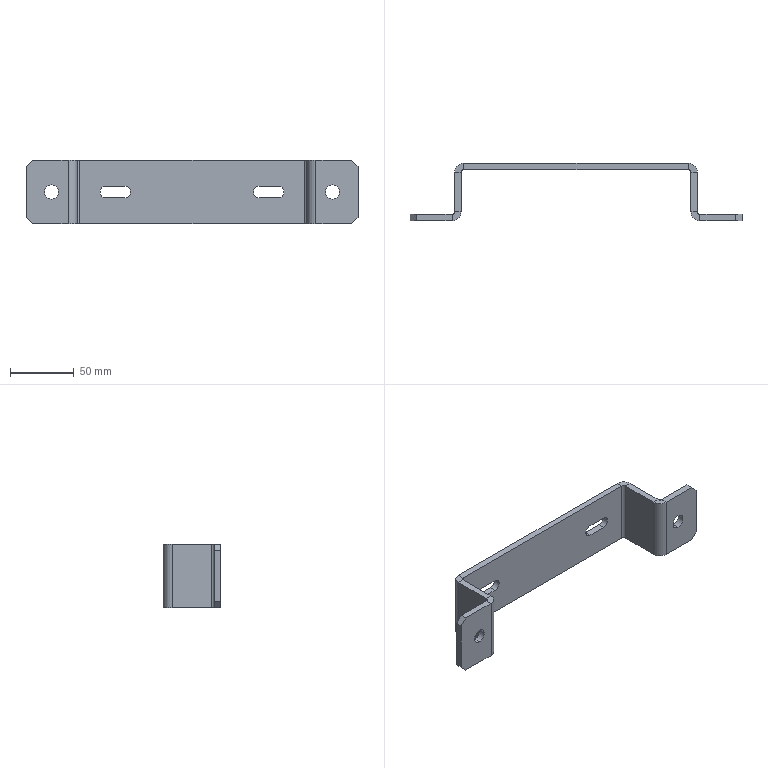Part | SolidWorks | features ICE 2, Chamfer 1, FlatPattern 1, SMBaseFlange 1, SheetMetal 1 | 1 solid | 54 faces | box 260 x 45 x 50 mm | volume 79882 mm3 | plane 38 | cylinder 16 | commonest cylinder face diameters 4 x4 9 x4 11 x4 14 x4
STEP:
#1=CARTESIAN_POINT('',(110.,0.,19.5));
#2=VERTEX_POINT('',#1);
#3=CARTESIAN_POINT('',(110.,0.,30.5));
#4=VERTEX_POINT('',#3);
#5=CARTESIAN_POINT('',(110.,0.,25.));
#6=DIRECTION('',(0.,1.,0.));
#7=DIRECTION('',(0.,0.,1.));
#8=AXIS2_PLACEMENT_3D('',#5,#6,#7);
#9=CIRCLE('',#8,5.5);
#10=EDGE_CURVE('',#2,#4,#9,.T.);
#11=ORIENTED_EDGE('',*,*,#10,.F.);
#12=CARTESIAN_POINT('',(110.,5.,19.5));
#13=VERTEX_POINT('',#12);
#14=CARTESIAN_POINT('',(110.,0.,19.5));
#15=DIRECTION('',(0.,1.,0.));
#16=VECTOR('',#15,1000.);
#17=LINE('',#14,#16);
#18=EDGE_CURVE('',#2,#13,#17,.T.);
#19=ORIENTED_EDGE('',*,*,#18,.T.);
#20=CARTESIAN_POINT('',(110.,5.,30.5));
#21=VERTEX_POINT('',#20);
#22=CARTESIAN_POINT('',(110.,5.,25.));
#23=DIRECTION('',(0.,1.,0.));
#24=DIRECTION('',(0.,0.,1.));
#25=AXIS2_PLACEMENT_3D('',#22,#23,#24);
#26=CIRCLE('',#25,5.5);
#27=EDGE_CURVE('',#13,#21,#26,.T.);
#28=ORIENTED_EDGE('',*,*,#27,.T.);
#29=CARTESIAN_POINT('',(110.,0.,30.5));
#30=DIRECTION('',(0.,1.,0.));
#31=VECTOR('',#30,1000.);
#32=LINE('',#29,#31);
#33=EDGE_CURVE('',#4,#21,#32,.T.);
#34=ORIENTED_EDGE('',*,*,#33,.F.);
#35=EDGE_LOOP('',(#11,#19,#28,#34));
#36=FACE_OUTER_BOUND('',#35,.T.);
#37=CARTESIAN_POINT('',(110.,0.,25.));
#38=DIRECTION('',(0.,1.,0.));
#39=DIRECTION('',(0.,0.,1.));
#40=AXIS2_PLACEMENT_3D('',#37,#38,#39);
#41=CYLINDRICAL_SURFACE('',#40,5.5);
#42=ADVANCED_FACE('',(#36),#41,.F.);
#43=CARTESIAN_POINT('',(-110.,0.,19.5));
#44=VERTEX_POINT('',#43);
#45=CARTESIAN_POINT('',(-110.,0.,30.5));
#46=VERTEX_POINT('',#45);
#47=CARTESIAN_POINT('',(-110.,0.,25.));
#48=DIRECTION('',(0.,1.,0.));
#49=DIRECTION('',(0.,0.,1.));
#50=AXIS2_PLACEMENT_3D('',#47,#48,#49);
#51=CIRCLE('',#50,5.5);
#52=EDGE_CURVE('',#44,#46,#51,.T.);
#53=ORIENTED_EDGE('',*,*,#52,.F.);
#54=CARTESIAN_POINT('',(-110.,5.,19.5));
#55=VERTEX_POINT('',#54);
#56=CARTESIAN_POINT('',(-110.,0.,19.5));
#57=DIRECTION('',(0.,1.,0.));
#58=VECTOR('',#57,1000.);
#59=LINE('',#56,#58);
#60=EDGE_CURVE('',#44,#55,#59,.T.);
#61=ORIENTED_EDGE('',*,*,#60,.T.);
#62=CARTESIAN_POINT('',(-110.,5.,30.5));
#63=VERTEX_POINT('',#62);
#64=CARTESIAN_POINT('',(-110.,5.,25.));
#65=DIRECTION('',(0.,1.,0.));
#66=DIRECTION('',(0.,0.,1.));
#67=AXIS2_PLACEMENT_3D('',#64,#65,#66);
#68=CIRCLE('',#67,5.5);
#69=EDGE_CURVE('',#55,#63,#68,.T.);
#70=ORIENTED_EDGE('',*,*,#69,.T.);
#71=CARTESIAN_POINT('',(-110.,0.,30.5));
#72=DIRECTION('',(0.,1.,0.));
#73=VECTOR('',#72,1000.);
#74=LINE('',#71,#73);
#75=EDGE_CURVE('',#46,#63,#74,.T.);
#76=ORIENTED_EDGE('',*,*,#75,.F.);
#77=EDGE_LOOP('',(#53,#61,#70,#76));
#78=FACE_OUTER_BOUND('',#77,.T.);
#79=CARTESIAN_POINT('',(-110.,0.,25.));
#80=DIRECTION('',(0.,1.,0.));
#81=DIRECTION('',(0.,0.,1.));
#82=AXIS2_PLACEMENT_3D('',#79,#80,#81);
#83=CYLINDRICAL_SURFACE('',#82,5.5);
#84=ADVANCED_FACE('',(#78),#83,.F.);
#85=CARTESIAN_POINT('',(-97.,0.,50.));
#86=VERTEX_POINT('',#85);
#87=CARTESIAN_POINT('',(-97.,5.,50.));
#88=VERTEX_POINT('',#87);
#89=CARTESIAN_POINT('',(-97.,0.,50.));
#90=DIRECTION('',(0.,1.,0.));
#91=VECTOR('',#90,1000.);
#92=LINE('',#89,#91);
#93=EDGE_CURVE('',#86,#88,#92,.T.);
#94=ORIENTED_EDGE('',*,*,#93,.F.);
#95=CARTESIAN_POINT('',(-90.,7.,50.));
#96=VERTEX_POINT('',#95);
#97=CARTESIAN_POINT('',(-97.,7.,50.));
#98=DIRECTION('',(0.,0.,1.));
#99=DIRECTION('',(-1.,0.,0.));
#100=AXIS2_PLACEMENT_3D('',#97,#98,#99);
#101=CIRCLE('',#100,7.);
#102=EDGE_CURVE('',#86,#96,#101,.T.);
#103=ORIENTED_EDGE('',*,*,#102,.T.);
#104=CARTESIAN_POINT('',(-95.,7.,50.));
#105=VERTEX_POINT('',#104);
#106=CARTESIAN_POINT('',(-95.,7.,50.));
#107=DIRECTION('',(1.,0.,0.));
#108=VECTOR('',#107,1000.);
#109=LINE('',#106,#108);
#110=EDGE_CURVE('',#105,#96,#109,.T.);
#111=ORIENTED_EDGE('',*,*,#110,.F.);
#112=CARTESIAN_POINT('',(-97.,7.,50.));
#113=DIRECTION('',(0.,0.,1.));
#114=DIRECTION('',(1.,0.,0.));
#115=AXIS2_PLACEMENT_3D('',#112,#113,#114);
#116=CIRCLE('',#115,2.);
#117=EDGE_CURVE('',#88,#105,#116,.T.);
#118=ORIENTED_EDGE('',*,*,#117,.F.);
#119=EDGE_LOOP('',(#94,#103,#111,#118));
#120=FACE_OUTER_BOUND('',#119,.T.);
#121=CARTESIAN_POINT('',(-97.,0.,50.));
#122=DIRECTION('',(0.,0.,1.));
#123=DIRECTION('',(1.,0.,0.));
#124=AXIS2_PLACEMENT_3D('',#121,#122,#123);
#125=PLANE('',#124);
#126=ADVANCED_FACE('',(#120),#125,.T.);
#127=CARTESIAN_POINT('',(-125.,5.,50.));
#128=VERTEX_POINT('',#127);
#129=CARTESIAN_POINT('',(-130.,5.,50.));
#130=DIRECTION('',(1.,0.,0.));
#131=VECTOR('',#130,1000.);
#132=LINE('',#129,#131);
#133=EDGE_CURVE('',#128,#88,#132,.T.);
#134=ORIENTED_EDGE('',*,*,#133,.F.);
#135=CARTESIAN_POINT('',(-125.,0.,50.));
#136=VERTEX_POINT('',#135);
#137=CARTESIAN_POINT('',(-125.,7.,50.));
#138=DIRECTION('',(0.,-1.,0.));
#139=VECTOR('',#138,1000.);
#140=LINE('',#137,#139);
#141=EDGE_CURVE('',#128,#136,#140,.T.);
#142=ORIENTED_EDGE('',*,*,#141,.T.);
#143=CARTESIAN_POINT('',(-130.,0.,50.));
#144=DIRECTION('',(1.,0.,0.));
#145=VECTOR('',#144,1000.);
#146=LINE('',#143,#145);
#147=EDGE_CURVE('',#136,#86,#146,.T.);
#148=ORIENTED_EDGE('',*,*,#147,.T.);
#149=ORIENTED_EDGE('',*,*,#93,.T.);
#150=EDGE_LOOP('',(#134,#142,#148,#149));
#151=FACE_OUTER_BOUND('',#150,.T.);
#152=CARTESIAN_POINT('',(-95.,7.,50.));
#153=DIRECTION('',(0.,0.,1.));
#154=DIRECTION('',(1.,0.,0.));
#155=AXIS2_PLACEMENT_3D('',#152,#153,#154);
#156=PLANE('',#155);
#157=ADVANCED_FACE('',(#151),#156,.T.);
#158=CARTESIAN_POINT('',(-90.,7.,0.));
#159=VERTEX_POINT('',#158);
#160=CARTESIAN_POINT('',(-95.,7.,0.));
#161=VERTEX_POINT('',#160);
#162=CARTESIAN_POINT('',(-90.,7.,0.));
#163=DIRECTION('',(-1.,0.,0.));
#164=VECTOR('',#163,1000.);
#165=LINE('',#162,#164);
#166=EDGE_CURVE('',#159,#161,#165,.T.);
#167=ORIENTED_EDGE('',*,*,#166,.F.);
#168=CARTESIAN_POINT('',(-97.,0.,0.));
#169=VERTEX_POINT('',#168);
#170=CARTESIAN_POINT('',(-97.,7.,0.));
#171=DIRECTION('',(0.,0.,1.));
#172=DIRECTION('',(-1.,0.,0.));
#173=AXIS2_PLACEMENT_3D('',#170,#171,#172);
#174=CIRCLE('',#173,7.);
#175=EDGE_CURVE('',#169,#159,#174,.T.);
#176=ORIENTED_EDGE('',*,*,#175,.F.);
#177=CARTESIAN_POINT('',(-97.,5.,0.));
#178=VERTEX_POINT('',#177);
#179=CARTESIAN_POINT('',(-97.,5.,0.));
#180=DIRECTION('',(0.,-1.,0.));
#181=VECTOR('',#180,1000.);
#182=LINE('',#179,#181);
#183=EDGE_CURVE('',#178,#169,#182,.T.);
#184=ORIENTED_EDGE('',*,*,#183,.F.);
#185=CARTESIAN_POINT('',(-97.,7.,0.));
#186=DIRECTION('',(0.,0.,1.));
#187=DIRECTION('',(1.,0.,0.));
#188=AXIS2_PLACEMENT_3D('',#185,#186,#187);
#189=CIRCLE('',#188,2.);
#190=EDGE_CURVE('',#178,#161,#189,.T.);
#191=ORIENTED_EDGE('',*,*,#190,.T.);
#192=EDGE_LOOP('',(#167,#176,#184,#191));
#193=FACE_OUTER_BOUND('',#192,.T.);
#194=CARTESIAN_POINT('',(-90.,7.,0.));
#195=DIRECTION('',(0.,0.,-1.));
#196=DIRECTION('',(-1.,0.,0.));
#197=AXIS2_PLACEMENT_3D('',#194,#195,#196);
#198=PLANE('',#197);
#199=ADVANCED_FACE('',(#193),#198,.T.);
#200=CARTESIAN_POINT('',(-90.,38.,0.));
#201=VERTEX_POINT('',#200);
#202=CARTESIAN_POINT('',(-90.,0.,0.));
#203=DIRECTION('',(0.,1.,0.));
#204=VECTOR('',#203,1000.);
#205=LINE('',#202,#204);
#206=EDGE_CURVE('',#159,#201,#205,.T.);
#207=ORIENTED_EDGE('',*,*,#206,.F.);
#208=ORIENTED_EDGE('',*,*,#166,.T.);
#209=CARTESIAN_POINT('',(-95.,38.,0.));
#210=VERTEX_POINT('',#209);
#211=CARTESIAN_POINT('',(-95.,0.,0.));
#212=DIRECTION('',(0.,1.,0.));
#213=VECTOR('',#212,1000.);
#214=LINE('',#211,#213);
#215=EDGE_CURVE('',#161,#210,#214,.T.);
#216=ORIENTED_EDGE('',*,*,#215,.T.);
#217=CARTESIAN_POINT('',(-95.,38.,0.));
#218=DIRECTION('',(1.,0.,0.));
#219=VECTOR('',#218,1000.);
#220=LINE('',#217,#219);
#221=EDGE_CURVE('',#210,#201,#220,.T.);
#222=ORIENTED_EDGE('',*,*,#221,.T.);
#223=EDGE_LOOP('',(#207,#208,#216,#222));
#224=FACE_OUTER_BOUND('',#223,.T.);
#225=CARTESIAN_POINT('',(-97.,5.,0.));
#226=DIRECTION('',(0.,0.,-1.));
#227=DIRECTION('',(-1.,0.,0.));
#228=AXIS2_PLACEMENT_3D('',#225,#226,#227);
#229=PLANE('',#228);
#230=ADVANCED_FACE('',(#224),#229,.T.);
#231=CARTESIAN_POINT('',(-90.,38.,50.));
#232=VERTEX_POINT('',#231);
#233=CARTESIAN_POINT('',(-95.,38.,50.));
#234=VERTEX_POINT('',#233);
#235=CARTESIAN_POINT('',(-90.,38.,50.));
#236=DIRECTION('',(-1.,0.,0.));
#237=VECTOR('',#236,1000.);
#238=LINE('',#235,#237);
#239=EDGE_CURVE('',#232,#234,#238,.T.);
#240=ORIENTED_EDGE('',*,*,#239,.F.);
#241=CARTESIAN_POINT('',(-88.,40.,50.));
#242=VERTEX_POINT('',#241);
#243=CARTESIAN_POINT('',(-88.,38.,50.));
#244=DIRECTION('',(0.,0.,-1.));
#245=DIRECTION('',(1.,0.,0.));
#246=AXIS2_PLACEMENT_3D('',#243,#244,#245);
#247=CIRCLE('',#246,2.);
#248=EDGE_CURVE('',#232,#242,#247,.T.);
#249=ORIENTED_EDGE('',*,*,#248,.T.);
#250=CARTESIAN_POINT('',(-88.,45.,50.));
#251=VERTEX_POINT('',#250);
#252=CARTESIAN_POINT('',(-88.,45.,50.));
#253=DIRECTION('',(0.,-1.,0.));
#254=VECTOR('',#253,1000.);
#255=LINE('',#252,#254);
#256=EDGE_CURVE('',#251,#242,#255,.T.);
#257=ORIENTED_EDGE('',*,*,#256,.F.);
#258=CARTESIAN_POINT('',(-88.,38.,50.));
#259=DIRECTION('',(0.,0.,-1.));
#260=DIRECTION('',(1.,0.,0.));
#261=AXIS2_PLACEMENT_3D('',#258,#259,#260);
#262=CIRCLE('',#261,7.);
#263=EDGE_CURVE('',#234,#251,#262,.T.);
#264=ORIENTED_EDGE('',*,*,#263,.F.);
#265=EDGE_LOOP('',(#240,#249,#257,#264));
#266=FACE_OUTER_BOUND('',#265,.T.);
#267=CARTESIAN_POINT('',(-90.,38.,50.));
#268=DIRECTION('',(0.,0.,1.));
#269=DIRECTION('',(1.,0.,0.));
#270=AXIS2_PLACEMENT_3D('',#267,#268,#269);
#271=PLANE('',#270);
#272=ADVANCED_FACE('',(#266),#271,.T.);
#273=CARTESIAN_POINT('',(-90.,0.,50.));
#274=DIRECTION('',(0.,1.,0.));
#275=VECTOR('',#274,1000.);
#276=LINE('',#273,#275);
#277=EDGE_CURVE('',#96,#232,#276,.T.);
#278=ORIENTED_EDGE('',*,*,#277,.T.);
#279=ORIENTED_EDGE('',*,*,#239,.T.);
#280=CARTESIAN_POINT('',(-95.,0.,50.));
#281=DIRECTION('',(0.,1.,0.));
#282=VECTOR('',#281,1000.);
#283=LINE('',#280,#282);
#284=EDGE_CURVE('',#105,#234,#283,.T.);
#285=ORIENTED_EDGE('',*,*,#284,.F.);
#286=ORIENTED_EDGE('',*,*,#110,.T.);
#287=EDGE_LOOP('',(#278,#279,#285,#286));
#288=FACE_OUTER_BOUND('',#287,.T.);
#289=CARTESIAN_POINT('',(-88.,45.,50.));
#290=DIRECTION('',(0.,0.,1.));
#291=DIRECTION('',(1.,0.,0.));
#292=AXIS2_PLACEMENT_3D('',#289,#290,#291);
#293=PLANE('',#292);
#294=ADVANCED_FACE('',(#288),#293,.T.);
#295=CARTESIAN_POINT('',(-88.,40.,0.));
#296=VERTEX_POINT('',#295);
#297=CARTESIAN_POINT('',(-88.,45.,0.));
#298=VERTEX_POINT('',#297);
#299=CARTESIAN_POINT('',(-88.,40.,0.));
#300=DIRECTION('',(0.,1.,0.));
#301=VECTOR('',#300,1000.);
#302=LINE('',#299,#301);
#303=EDGE_CURVE('',#296,#298,#302,.T.);
#304=ORIENTED_EDGE('',*,*,#303,.F.);
#305=CARTESIAN_POINT('',(-88.,38.,0.));
#306=DIRECTION('',(0.,0.,-1.));
#307=DIRECTION('',(1.,0.,0.));
#308=AXIS2_PLACEMENT_3D('',#305,#306,#307);
#309=CIRCLE('',#308,2.);
#310=EDGE_CURVE('',#201,#296,#309,.T.);
#311=ORIENTED_EDGE('',*,*,#310,.F.);
#312=ORIENTED_EDGE('',*,*,#221,.F.);
#313=CARTESIAN_POINT('',(-88.,38.,0.));
#314=DIRECTION('',(0.,0.,-1.));
#315=DIRECTION('',(1.,0.,0.));
#316=AXIS2_PLACEMENT_3D('',#313,#314,#315);
#317=CIRCLE('',#316,7.);
#318=EDGE_CURVE('',#210,#298,#317,.T.);
#319=ORIENTED_EDGE('',*,*,#318,.T.);
#320=EDGE_LOOP('',(#304,#311,#312,#319));
#321=FACE_OUTER_BOUND('',#320,.T.);
#322=CARTESIAN_POINT('',(-88.,40.,0.));
#323=DIRECTION('',(0.,0.,-1.));
#324=DIRECTION('',(-1.,0.,0.));
#325=AXIS2_PLACEMENT_3D('',#322,#323,#324);
#326=PLANE('',#325);
#327=ADVANCED_FACE('',(#321),#326,.T.);
#328=CARTESIAN_POINT('',(88.,40.,0.));
#329=VERTEX_POINT('',#328);
#330=CARTESIAN_POINT('',(-90.,40.,0.));
#331=DIRECTION('',(1.,0.,0.));
#332=VECTOR('',#331,1000.);
#333=LINE('',#330,#332);
#334=EDGE_CURVE('',#296,#329,#333,.T.);
#335=ORIENTED_EDGE('',*,*,#334,.F.);
#336=ORIENTED_EDGE('',*,*,#303,.T.);
#337=CARTESIAN_POINT('',(88.,45.,0.));
#338=VERTEX_POINT('',#337);
#339=CARTESIAN_POINT('',(-90.,45.,0.));
#340=DIRECTION('',(1.,0.,0.));
#341=VECTOR('',#340,1000.);
#342=LINE('',#339,#341);
#343=EDGE_CURVE('',#298,#338,#342,.T.);
#344=ORIENTED_EDGE('',*,*,#343,.T.);
#345=CARTESIAN_POINT('',(88.,45.,0.));
#346=DIRECTION('',(0.,-1.,0.));
#347=VECTOR('',#346,1000.);
#348=LINE('',#345,#347);
#349=EDGE_CURVE('',#338,#329,#348,.T.);
#350=ORIENTED_EDGE('',*,*,#349,.T.);
#351=EDGE_LOOP('',(#335,#336,#344,#350));
#352=FACE_OUTER_BOUND('',#351,.T.);
#353=CARTESIAN_POINT('',(-95.,38.,0.));
#354=DIRECTION('',(0.,0.,-1.));
#355=DIRECTION('',(-1.,0.,0.));
#356=AXIS2_PLACEMENT_3D('',#353,#354,#355);
#357=PLANE('',#356);
#358=ADVANCED_FACE('',(#352),#357,.T.);
#359=CARTESIAN_POINT('',(88.,40.,50.));
#360=VERTEX_POINT('',#359);
#361=CARTESIAN_POINT('',(88.,45.,50.));
#362=VERTEX_POINT('',#361);
#363=CARTESIAN_POINT('',(88.,40.,50.));
#364=DIRECTION('',(0.,1.,0.));
#365=VECTOR('',#364,1000.);
#366=LINE('',#363,#365);
#367=EDGE_CURVE('',#360,#362,#366,.T.);
#368=ORIENTED_EDGE('',*,*,#367,.F.);
#369=CARTESIAN_POINT('',(90.,38.,50.));
#370=VERTEX_POINT('',#369);
#371=CARTESIAN_POINT('',(88.,38.,50.));
#372=DIRECTION('',(0.,0.,-1.));
#373=DIRECTION('',(1.,0.,0.));
#374=AXIS2_PLACEMENT_3D('',#371,#372,#373);
#375=CIRCLE('',#374,2.);
#376=EDGE_CURVE('',#360,#370,#375,.T.);
#377=ORIENTED_EDGE('',*,*,#376,.T.);
#378=CARTESIAN_POINT('',(95.,38.,50.));
#379=VERTEX_POINT('',#378);
#380=CARTESIAN_POINT('',(95.,38.,50.));
#381=DIRECTION('',(-1.,0.,0.));
#382=VECTOR('',#381,1000.);
#383=LINE('',#380,#382);
#384=EDGE_CURVE('',#379,#370,#383,.T.);
#385=ORIENTED_EDGE('',*,*,#384,.F.);
#386=CARTESIAN_POINT('',(88.,38.,50.));
#387=DIRECTION('',(0.,0.,-1.));
#388=DIRECTION('',(1.,0.,0.));
#389=AXIS2_PLACEMENT_3D('',#386,#387,#388);
#390=CIRCLE('',#389,7.);
#391=EDGE_CURVE('',#362,#379,#390,.T.);
#392=ORIENTED_EDGE('',*,*,#391,.F.);
#393=EDGE_LOOP('',(#368,#377,#385,#392));
#394=FACE_OUTER_BOUND('',#393,.T.);
#395=CARTESIAN_POINT('',(88.,40.,50.));
#396=DIRECTION('',(0.,0.,1.));
#397=DIRECTION('',(1.,0.,0.));
#398=AXIS2_PLACEMENT_3D('',#395,#396,#397);
#399=PLANE('',#398);
#400=ADVANCED_FACE('',(#394),#399,.T.);
#401=CARTESIAN_POINT('',(-90.,40.,50.));
#402=DIRECTION('',(1.,0.,0.));
#403=VECTOR('',#402,1000.);
#404=LINE('',#401,#403);
#405=EDGE_CURVE('',#242,#360,#404,.T.);
#406=ORIENTED_EDGE('',*,*,#405,.T.);
#407=ORIENTED_EDGE('',*,*,#367,.T.);
#408=CARTESIAN_POINT('',(-90.,45.,50.));
#409=DIRECTION('',(1.,0.,0.));
#410=VECTOR('',#409,1000.);
#411=LINE('',#408,#410);
#412=EDGE_CURVE('',#251,#362,#411,.T.);
#413=ORIENTED_EDGE('',*,*,#412,.F.);
#414=ORIENTED_EDGE('',*,*,#256,.T.);
#415=EDGE_LOOP('',(#406,#407,#413,#414));
#416=FACE_OUTER_BOUND('',#415,.T.);
#417=CARTESIAN_POINT('',(95.,38.,50.));
#418=DIRECTION('',(0.,0.,1.));
#419=DIRECTION('',(1.,0.,0.));
#420=AXIS2_PLACEMENT_3D('',#417,#418,#419);
#421=PLANE('',#420);
#422=ADVANCED_FACE('',(#416),#421,.T.);
#423=CARTESIAN_POINT('',(90.,38.,0.));
#424=VERTEX_POINT('',#423);
#425=CARTESIAN_POINT('',(95.,38.,0.));
#426=VERTEX_POINT('',#425);
#427=CARTESIAN_POINT('',(90.,38.,0.));
#428=DIRECTION('',(1.,0.,0.));
#429=VECTOR('',#428,1000.);
#430=LINE('',#427,#429);
#431=EDGE_CURVE('',#424,#426,#430,.T.);
#432=ORIENTED_EDGE('',*,*,#431,.F.);
#433=CARTESIAN_POINT('',(88.,38.,0.));
#434=DIRECTION('',(0.,0.,-1.));
#435=DIRECTION('',(1.,0.,0.));
#436=AXIS2_PLACEMENT_3D('',#433,#434,#435);
#437=CIRCLE('',#436,2.);
#438=EDGE_CURVE('',#329,#424,#437,.T.);
#439=ORIENTED_EDGE('',*,*,#438,.F.);
#440=ORIENTED_EDGE('',*,*,#349,.F.);
#441=CARTESIAN_POINT('',(88.,38.,0.));
#442=DIRECTION('',(0.,0.,-1.));
#443=DIRECTION('',(1.,0.,0.));
#444=AXIS2_PLACEMENT_3D('',#441,#442,#443);
#445=CIRCLE('',#444,7.);
#446=EDGE_CURVE('',#338,#426,#445,.T.);
#447=ORIENTED_EDGE('',*,*,#446,.T.);
#448=EDGE_LOOP('',(#432,#439,#440,#447));
#449=FACE_OUTER_BOUND('',#448,.T.);
#450=CARTESIAN_POINT('',(90.,38.,0.));
#451=DIRECTION('',(0.,0.,-1.));
#452=DIRECTION('',(-1.,0.,0.));
#453=AXIS2_PLACEMENT_3D('',#450,#451,#452);
#454=PLANE('',#453);
#455=ADVANCED_FACE('',(#449),#454,.T.);
#456=CARTESIAN_POINT('',(90.,7.,0.));
#457=VERTEX_POINT('',#456);
#458=CARTESIAN_POINT('',(90.,40.,0.));
#459=DIRECTION('',(0.,-1.,0.));
#460=VECTOR('',#459,1000.);
#461=LINE('',#458,#460);
#462=EDGE_CURVE('',#424,#457,#461,.T.);
#463=ORIENTED_EDGE('',*,*,#462,.F.);
#464=ORIENTED_EDGE('',*,*,#431,.T.);
#465=CARTESIAN_POINT('',(95.,7.,0.));
#466=VERTEX_POINT('',#465);
#467=CARTESIAN_POINT('',(95.,40.,0.));
#468=DIRECTION('',(0.,-1.,0.));
#469=VECTOR('',#468,1000.);
#470=LINE('',#467,#469);
#471=EDGE_CURVE('',#426,#466,#470,.T.);
#472=ORIENTED_EDGE('',*,*,#471,.T.);
#473=CARTESIAN_POINT('',(95.,7.,0.));
#474=DIRECTION('',(-1.,0.,0.));
#475=VECTOR('',#474,1000.);
#476=LINE('',#473,#475);
#477=EDGE_CURVE('',#466,#457,#476,.T.);
#478=ORIENTED_EDGE('',*,*,#477,.T.);
#479=EDGE_LOOP('',(#463,#464,#472,#478));
#480=FACE_OUTER_BOUND('',#479,.T.);
#481=CARTESIAN_POINT('',(88.,45.,0.));
#482=DIRECTION('',(0.,0.,-1.));
#483=DIRECTION('',(-1.,0.,0.));
#484=AXIS2_PLACEMENT_3D('',#481,#482,#483);
#485=PLANE('',#484);
#486=ADVANCED_FACE('',(#480),#485,.T.);
#487=CARTESIAN_POINT('',(90.,7.,50.));
#488=VERTEX_POINT('',#487);
#489=CARTESIAN_POINT('',(95.,7.,50.));
#490=VERTEX_POINT('',#489);
#491=CARTESIAN_POINT('',(90.,7.,50.));
#492=DIRECTION('',(1.,0.,0.));
#493=VECTOR('',#492,1000.);
#494=LINE('',#491,#493);
#495=EDGE_CURVE('',#488,#490,#494,.T.);
#496=ORIENTED_EDGE('',*,*,#495,.F.);
#497=CARTESIAN_POINT('',(97.,0.,50.));
#498=VERTEX_POINT('',#497);
#499=CARTESIAN_POINT('',(97.,7.,50.));
#500=DIRECTION('',(0.,0.,1.));
#501=DIRECTION('',(-1.,0.,0.));
#502=AXIS2_PLACEMENT_3D('',#499,#500,#501);
#503=CIRCLE('',#502,7.);
#504=EDGE_CURVE('',#488,#498,#503,.T.);
#505=ORIENTED_EDGE('',*,*,#504,.T.);
#506=CARTESIAN_POINT('',(97.,5.,50.));
#507=VERTEX_POINT('',#506);
#508=CARTESIAN_POINT('',(97.,5.,50.));
#509=DIRECTION('',(0.,-1.,0.));
#510=VECTOR('',#509,1000.);
#511=LINE('',#508,#510);
#512=EDGE_CURVE('',#507,#498,#511,.T.);
#513=ORIENTED_EDGE('',*,*,#512,.F.);
#514=CARTESIAN_POINT('',(97.,7.,50.));
#515=DIRECTION('',(0.,0.,1.));
#516=DIRECTION('',(1.,0.,0.));
#517=AXIS2_PLACEMENT_3D('',#514,#515,#516);
#518=CIRCLE('',#517,2.);
#519=EDGE_CURVE('',#490,#507,#518,.T.);
#520=ORIENTED_EDGE('',*,*,#519,.F.);
#521=EDGE_LOOP('',(#496,#505,#513,#520));
#522=FACE_OUTER_BOUND('',#521,.T.);
#523=CARTESIAN_POINT('',(90.,7.,50.));
#524=DIRECTION('',(0.,0.,1.));
#525=DIRECTION('',(1.,0.,0.));
#526=AXIS2_PLACEMENT_3D('',#523,#524,#525);
#527=PLANE('',#526);
#528=ADVANCED_FACE('',(#522),#527,.T.);
#529=CARTESIAN_POINT('',(90.,40.,50.));
#530=DIRECTION('',(0.,-1.,0.));
#531=VECTOR('',#530,1000.);
#532=LINE('',#529,#531);
#533=EDGE_CURVE('',#370,#488,#532,.T.);
#534=ORIENTED_EDGE('',*,*,#533,.T.);
#535=ORIENTED_EDGE('',*,*,#495,.T.);
#536=CARTESIAN_POINT('',(95.,40.,50.));
#537=DIRECTION('',(0.,-1.,0.));
#538=VECTOR('',#537,1000.);
#539=LINE('',#536,#538);
#540=EDGE_CURVE('',#379,#490,#539,.T.);
#541=ORIENTED_EDGE('',*,*,#540,.F.);
#542=ORIENTED_EDGE('',*,*,#384,.T.);
#543=EDGE_LOOP('',(#534,#535,#541,#542));
#544=FACE_OUTER_BOUND('',#543,.T.);
#545=CARTESIAN_POINT('',(97.,5.,50.));
#546=DIRECTION('',(0.,0.,1.));
#547=DIRECTION('',(1.,0.,0.));
#548=AXIS2_PLACEMENT_3D('',#545,#546,#547);
#549=PLANE('',#548);
#550=ADVANCED_FACE('',(#544),#549,.T.);
#551=CARTESIAN_POINT('',(97.,0.,0.));
#552=VERTEX_POINT('',#551);
#553=CARTESIAN_POINT('',(97.,5.,0.));
#554=VERTEX_POINT('',#553);
#555=CARTESIAN_POINT('',(97.,0.,0.));
#556=DIRECTION('',(0.,1.,0.));
#557=VECTOR('',#556,1000.);
#558=LINE('',#555,#557);
#559=EDGE_CURVE('',#552,#554,#558,.T.);
#560=ORIENTED_EDGE('',*,*,#559,.F.);
#561=CARTESIAN_POINT('',(97.,7.,0.));
#562=DIRECTION('',(0.,0.,1.));
#563=DIRECTION('',(-1.,0.,0.));
#564=AXIS2_PLACEMENT_3D('',#561,#562,#563);
#565=CIRCLE('',#564,7.);
#566=EDGE_CURVE('',#457,#552,#565,.T.);
#567=ORIENTED_EDGE('',*,*,#566,.F.);
#568=ORIENTED_EDGE('',*,*,#477,.F.);
#569=CARTESIAN_POINT('',(97.,7.,0.));
#570=DIRECTION('',(0.,0.,1.));
#571=DIRECTION('',(1.,0.,0.));
#572=AXIS2_PLACEMENT_3D('',#569,#570,#571);
#573=CIRCLE('',#572,2.);
#574=EDGE_CURVE('',#466,#554,#573,.T.);
#575=ORIENTED_EDGE('',*,*,#574,.T.);
#576=EDGE_LOOP('',(#560,#567,#568,#575));
#577=FACE_OUTER_BOUND('',#576,.T.);
#578=CARTESIAN_POINT('',(97.,0.,0.));
#579=DIRECTION('',(0.,0.,-1.));
#580=DIRECTION('',(-1.,0.,0.));
#581=AXIS2_PLACEMENT_3D('',#578,#579,#580);
#582=PLANE('',#581);
#583=ADVANCED_FACE('',(#577),#582,.T.);
#584=CARTESIAN_POINT('',(125.,5.,0.));
#585=VERTEX_POINT('',#584);
#586=CARTESIAN_POINT('',(90.,5.,0.));
#587=DIRECTION('',(1.,0.,0.));
#588=VECTOR('',#587,1000.);
#589=LINE('',#586,#588);
#590=EDGE_CURVE('',#554,#585,#589,.T.);
#591=ORIENTED_EDGE('',*,*,#590,.T.);
#592=CARTESIAN_POINT('',(125.,0.,0.));
#593=VERTEX_POINT('',#592);
#594=CARTESIAN_POINT('',(125.,7.,0.));
#595=DIRECTION('',(0.,-1.,0.));
#596=VECTOR('',#595,1000.);
#597=LINE('',#594,#596);
#598=EDGE_CURVE('',#585,#593,#597,.T.);
#599=ORIENTED_EDGE('',*,*,#598,.T.);
#600=CARTESIAN_POINT('',(90.,0.,0.));
#601=DIRECTION('',(1.,0.,0.));
#602=VECTOR('',#601,1000.);
#603=LINE('',#600,#602);
#604=EDGE_CURVE('',#552,#593,#603,.T.);
#605=ORIENTED_EDGE('',*,*,#604,.F.);
#606=ORIENTED_EDGE('',*,*,#559,.T.);
#607=EDGE_LOOP('',(#591,#599,#605,#606));
#608=FACE_OUTER_BOUND('',#607,.T.);
#609=CARTESIAN_POINT('',(95.,7.,0.));
#610=DIRECTION('',(0.,0.,-1.));
#611=DIRECTION('',(-1.,0.,0.));
#612=AXIS2_PLACEMENT_3D('',#609,#610,#611);
#613=PLANE('',#612);
#614=ADVANCED_FACE('',(#608),#613,.T.);
#615=CARTESIAN_POINT('',(110.,0.,25.));
#616=DIRECTION('',(0.,1.,0.));
#617=DIRECTION('',(0.,0.,1.));
#618=AXIS2_PLACEMENT_3D('',#615,#616,#617);
#619=CIRCLE('',#618,5.5);
#620=EDGE_CURVE('',#4,#2,#619,.T.);
#621=ORIENTED_EDGE('',*,*,#620,.T.);
#622=ORIENTED_EDGE('',*,*,#10,.T.);
#623=EDGE_LOOP('',(#621,#622));
#624=FACE_BOUND('',#623,.T.);
#625=ORIENTED_EDGE('',*,*,#604,.T.);
#626=CARTESIAN_POINT('',(130.,0.,5.));
#627=VERTEX_POINT('',#626);
#628=CARTESIAN_POINT('',(125.,0.,0.));
#629=DIRECTION('',(0.7071,0.,0.7071));
#630=VECTOR('',#629,1000.);
#631=LINE('',#628,#630);
#632=EDGE_CURVE('',#593,#627,#631,.T.);
#633=ORIENTED_EDGE('',*,*,#632,.T.);
#634=CARTESIAN_POINT('',(130.,0.,45.));
#635=VERTEX_POINT('',#634);
#636=CARTESIAN_POINT('',(130.,0.,50.));
#637=DIRECTION('',(0.,0.,-1.));
#638=VECTOR('',#637,1000.);
#639=LINE('',#636,#638);
#640=EDGE_CURVE('',#635,#627,#639,.T.);
#641=ORIENTED_EDGE('',*,*,#640,.F.);
#642=CARTESIAN_POINT('',(125.,0.,50.));
#643=VERTEX_POINT('',#642);
#644=CARTESIAN_POINT('',(130.,0.,45.));
#645=DIRECTION('',(-0.7071,0.,0.7071));
#646=VECTOR('',#645,1000.);
#647=LINE('',#644,#646);
#648=EDGE_CURVE('',#635,#643,#647,.T.);
#649=ORIENTED_EDGE('',*,*,#648,.T.);
#650=CARTESIAN_POINT('',(90.,0.,50.));
#651=DIRECTION('',(1.,0.,0.));
#652=VECTOR('',#651,1000.);
#653=LINE('',#650,#652);
#654=EDGE_CURVE('',#498,#643,#653,.T.);
#655=ORIENTED_EDGE('',*,*,#654,.F.);
#656=CARTESIAN_POINT('',(97.,0.,50.));
#657=DIRECTION('',(0.,0.,-1.));
#658=VECTOR('',#657,1000.);
#659=LINE('',#656,#658);
#660=EDGE_CURVE('',#498,#552,#659,.T.);
#661=ORIENTED_EDGE('',*,*,#660,.T.);
#662=EDGE_LOOP('',(#625,#633,#641,#649,#655,#661));
#663=FACE_OUTER_BOUND('',#662,.T.);
#664=CARTESIAN_POINT('',(90.,0.,50.));
#665=DIRECTION('',(0.,1.,0.));
#666=DIRECTION('',(-1.,0.,0.));
#667=AXIS2_PLACEMENT_3D('',#664,#665,#666);
#668=PLANE('',#667);
#669=ADVANCED_FACE('',(#624,#663),#668,.F.);
#670=ORIENTED_EDGE('',*,*,#640,.T.);
#671=CARTESIAN_POINT('',(130.,5.,5.));
#672=VERTEX_POINT('',#671);
#673=CARTESIAN_POINT('',(130.,5.,5.));
#674=DIRECTION('',(0.,1.,0.));
#675=VECTOR('',#674,1000.);
#676=LINE('',#673,#675);
#677=EDGE_CURVE('',#627,#672,#676,.T.);
#678=ORIENTED_EDGE('',*,*,#677,.T.);
#679=CARTESIAN_POINT('',(130.,5.,45.));
#680=VERTEX_POINT('',#679);
#681=CARTESIAN_POINT('',(130.,5.,50.));
#682=DIRECTION('',(0.,0.,-1.));
#683=VECTOR('',#682,1000.);
#684=LINE('',#681,#683);
#685=EDGE_CURVE('',#680,#672,#684,.T.);
#686=ORIENTED_EDGE('',*,*,#685,.F.);
#687=CARTESIAN_POINT('',(130.,5.,45.));
#688=DIRECTION('',(0.,-1.,0.));
#689=VECTOR('',#688,1000.);
#690=LINE('',#687,#689);
#691=EDGE_CURVE('',#680,#635,#690,.T.);
#692=ORIENTED_EDGE('',*,*,#691,.T.);
#693=EDGE_LOOP('',(#670,#678,#686,#692));
#694=FACE_OUTER_BOUND('',#693,.T.);
#695=CARTESIAN_POINT('',(130.,5.,50.));
#696=DIRECTION('',(1.,0.,0.));
#697=DIRECTION('',(0.,0.,-1.));
#698=AXIS2_PLACEMENT_3D('',#695,#696,#697);
#699=PLANE('',#698);
#700=ADVANCED_FACE('',(#694),#699,.T.);
#701=CARTESIAN_POINT('',(110.,5.,25.));
#702=DIRECTION('',(0.,1.,0.));
#703=DIRECTION('',(0.,0.,1.));
#704=AXIS2_PLACEMENT_3D('',#701,#702,#703);
#705=CIRCLE('',#704,5.5);
#706=EDGE_CURVE('',#21,#13,#705,.T.);
#707=ORIENTED_EDGE('',*,*,#706,.F.);
#708=ORIENTED_EDGE('',*,*,#27,.F.);
#709=EDGE_LOOP('',(#707,#708));
#710=FACE_BOUND('',#709,.T.);
#711=ORIENTED_EDGE('',*,*,#685,.T.);
#712=CARTESIAN_POINT('',(132.5,5.,7.5));
#713=DIRECTION('',(-0.7071,0.,-0.7071));
#714=VECTOR('',#713,1000.);
#715=LINE('',#712,#714);
#716=EDGE_CURVE('',#672,#585,#715,.T.);
#717=ORIENTED_EDGE('',*,*,#716,.T.);
#718=ORIENTED_EDGE('',*,*,#590,.F.);
#719=CARTESIAN_POINT('',(97.,5.,50.));
#720=DIRECTION('',(0.,0.,-1.));
#721=VECTOR('',#720,1000.);
#722=LINE('',#719,#721);
#723=EDGE_CURVE('',#507,#554,#722,.T.);
#724=ORIENTED_EDGE('',*,*,#723,.F.);
#725=CARTESIAN_POINT('',(125.,5.,50.));
#726=VERTEX_POINT('',#725);
#727=CARTESIAN_POINT('',(90.,5.,50.));
#728=DIRECTION('',(1.,0.,0.));
#729=VECTOR('',#728,1000.);
#730=LINE('',#727,#729);
#731=EDGE_CURVE('',#507,#726,#730,.T.);
#732=ORIENTED_EDGE('',*,*,#731,.T.);
#733=CARTESIAN_POINT('',(107.5,5.,67.5));
#734=DIRECTION('',(0.7071,0.,-0.7071));
#735=VECTOR('',#734,1000.);
#736=LINE('',#733,#735);
#737=EDGE_CURVE('',#726,#680,#736,.T.);
#738=ORIENTED_EDGE('',*,*,#737,.T.);
#739=EDGE_LOOP('',(#711,#717,#718,#724,#732,#738));
#740=FACE_OUTER_BOUND('',#739,.T.);
#741=CARTESIAN_POINT('',(90.,5.,50.));
#742=DIRECTION('',(0.,1.,0.));
#743=DIRECTION('',(-1.,0.,0.));
#744=AXIS2_PLACEMENT_3D('',#741,#742,#743);
#745=PLANE('',#744);
#746=ADVANCED_FACE('',(#710,#740),#745,.T.);
#747=ORIENTED_EDGE('',*,*,#574,.F.);
#748=CARTESIAN_POINT('',(95.,7.,50.));
#749=DIRECTION('',(0.,0.,-1.));
#750=VECTOR('',#749,1000.);
#751=LINE('',#748,#750);
#752=EDGE_CURVE('',#490,#466,#751,.T.);
#753=ORIENTED_EDGE('',*,*,#752,.F.);
#754=ORIENTED_EDGE('',*,*,#519,.T.);
#755=ORIENTED_EDGE('',*,*,#723,.T.);
#756=EDGE_LOOP('',(#747,#753,#754,#755));
#757=FACE_OUTER_BOUND('',#756,.T.);
#758=CARTESIAN_POINT('',(97.,7.,50.));
#759=DIRECTION('',(0.,0.,-1.));
#760=DIRECTION('',(-1.,0.,0.));
#761=AXIS2_PLACEMENT_3D('',#758,#759,#760);
#762=CYLINDRICAL_SURFACE('',#761,2.);
#763=ADVANCED_FACE('',(#757),#762,.F.);
#764=ORIENTED_EDGE('',*,*,#471,.F.);
#765=CARTESIAN_POINT('',(95.,38.,50.));
#766=DIRECTION('',(0.,0.,-1.));
#767=VECTOR('',#766,1000.);
#768=LINE('',#765,#767);
#769=EDGE_CURVE('',#379,#426,#768,.T.);
#770=ORIENTED_EDGE('',*,*,#769,.F.);
#771=ORIENTED_EDGE('',*,*,#540,.T.);
#772=ORIENTED_EDGE('',*,*,#752,.T.);
#773=EDGE_LOOP('',(#764,#770,#771,#772));
#774=FACE_OUTER_BOUND('',#773,.T.);
#775=CARTESIAN_POINT('',(95.,40.,50.));
#776=DIRECTION('',(1.,0.,0.));
#777=DIRECTION('',(0.,0.,-1.));
#778=AXIS2_PLACEMENT_3D('',#775,#776,#777);
#779=PLANE('',#778);
#780=ADVANCED_FACE('',(#774),#779,.T.);
#781=ORIENTED_EDGE('',*,*,#446,.F.);
#782=CARTESIAN_POINT('',(88.,45.,50.));
#783=DIRECTION('',(0.,0.,-1.));
#784=VECTOR('',#783,1000.);
#785=LINE('',#782,#784);
#786=EDGE_CURVE('',#362,#338,#785,.T.);
#787=ORIENTED_EDGE('',*,*,#786,.F.);
#788=ORIENTED_EDGE('',*,*,#391,.T.);
#789=ORIENTED_EDGE('',*,*,#769,.T.);
#790=EDGE_LOOP('',(#781,#787,#788,#789));
#791=FACE_OUTER_BOUND('',#790,.T.);
#792=CARTESIAN_POINT('',(88.,38.,50.));
#793=DIRECTION('',(0.,0.,-1.));
#794=DIRECTION('',(-1.,0.,0.));
#795=AXIS2_PLACEMENT_3D('',#792,#793,#794);
#796=CYLINDRICAL_SURFACE('',#795,7.);
#797=ADVANCED_FACE('',(#791),#796,.T.);
#798=CARTESIAN_POINT('',(-67.5,45.,20.5));
#799=VERTEX_POINT('',#798);
#800=CARTESIAN_POINT('',(-67.5,45.,29.5));
#801=VERTEX_POINT('',#800);
#802=CARTESIAN_POINT('',(-67.5,45.,25.));
#803=DIRECTION('',(0.,1.,0.));
#804=DIRECTION('',(0.,0.,1.));
#805=AXIS2_PLACEMENT_3D('',#802,#803,#804);
#806=CIRCLE('',#805,4.5);
#807=EDGE_CURVE('',#799,#801,#806,.T.);
#808=ORIENTED_EDGE('',*,*,#807,.F.);
#809=CARTESIAN_POINT('',(-52.5,45.,20.5));
#810=VERTEX_POINT('',#809);
#811=CARTESIAN_POINT('',(-67.5,45.,20.5));
#812=DIRECTION('',(-1.,0.,0.));
#813=VECTOR('',#812,1000.);
#814=LINE('',#811,#813);
#815=EDGE_CURVE('',#810,#799,#814,.T.);
#816=ORIENTED_EDGE('',*,*,#815,.F.);
#817=CARTESIAN_POINT('',(-52.5,45.,29.5));
#818=VERTEX_POINT('',#817);
#819=CARTESIAN_POINT('',(-52.5,45.,25.));
#820=DIRECTION('',(0.,1.,0.));
#821=DIRECTION('',(0.,0.,1.));
#822=AXIS2_PLACEMENT_3D('',#819,#820,#821);
#823=CIRCLE('',#822,4.5);
#824=EDGE_CURVE('',#818,#810,#823,.T.);
#825=ORIENTED_EDGE('',*,*,#824,.F.);
#826=CARTESIAN_POINT('',(-67.5,45.,29.5));
#827=DIRECTION('',(1.,0.,0.));
#828=VECTOR('',#827,1000.);
#829=LINE('',#826,#828);
#830=EDGE_CURVE('',#801,#818,#829,.T.);
#831=ORIENTED_EDGE('',*,*,#830,.F.);
#832=EDGE_LOOP('',(#808,#816,#825,#831));
#833=FACE_BOUND('',#832,.T.);
#834=CARTESIAN_POINT('',(52.5,45.,20.5));
#835=VERTEX_POINT('',#834);
#836=CARTESIAN_POINT('',(52.5,45.,29.5));
#837=VERTEX_POINT('',#836);
#838=CARTESIAN_POINT('',(52.5,45.,25.));
#839=DIRECTION('',(0.,1.,0.));
#840=DIRECTION('',(0.,0.,1.));
#841=AXIS2_PLACEMENT_3D('',#838,#839,#840);
#842=CIRCLE('',#841,4.5);
#843=EDGE_CURVE('',#835,#837,#842,.T.);
#844=ORIENTED_EDGE('',*,*,#843,.F.);
#845=CARTESIAN_POINT('',(67.5,45.,20.5));
#846=VERTEX_POINT('',#845);
#847=CARTESIAN_POINT('',(52.5,45.,20.5));
#848=DIRECTION('',(-1.,0.,0.));
#849=VECTOR('',#848,1000.);
#850=LINE('',#847,#849);
#851=EDGE_CURVE('',#846,#835,#850,.T.);
#852=ORIENTED_EDGE('',*,*,#851,.F.);
#853=CARTESIAN_POINT('',(67.5,45.,29.5));
#854=VERTEX_POINT('',#853);
#855=CARTESIAN_POINT('',(67.5,45.,25.));
#856=DIRECTION('',(0.,1.,0.));
#857=DIRECTION('',(0.,0.,1.));
#858=AXIS2_PLACEMENT_3D('',#855,#856,#857);
#859=CIRCLE('',#858,4.5);
#860=EDGE_CURVE('',#854,#846,#859,.T.);
#861=ORIENTED_EDGE('',*,*,#860,.F.);
#862=CARTESIAN_POINT('',(52.5,45.,29.5));
#863=DIRECTION('',(1.,0.,0.));
#864=VECTOR('',#863,1000.);
#865=LINE('',#862,#864);
#866=EDGE_CURVE('',#837,#854,#865,.T.);
#867=ORIENTED_EDGE('',*,*,#866,.F.);
#868=EDGE_LOOP('',(#844,#852,#861,#867));
#869=FACE_BOUND('',#868,.T.);
#870=ORIENTED_EDGE('',*,*,#343,.F.);
#871=CARTESIAN_POINT('',(-88.,45.,50.));
#872=DIRECTION('',(0.,0.,-1.));
#873=VECTOR('',#872,1000.);
#874=LINE('',#871,#873);
#875=EDGE_CURVE('',#251,#298,#874,.T.);
#876=ORIENTED_EDGE('',*,*,#875,.F.);
#877=ORIENTED_EDGE('',*,*,#412,.T.);
#878=ORIENTED_EDGE('',*,*,#786,.T.);
#879=EDGE_LOOP('',(#870,#876,#877,#878));
#880=FACE_OUTER_BOUND('',#879,.T.);
#881=CARTESIAN_POINT('',(-90.,45.,50.));
#882=DIRECTION('',(0.,1.,0.));
#883=DIRECTION('',(0.,0.,1.));
#884=AXIS2_PLACEMENT_3D('',#881,#882,#883);
#885=PLANE('',#884);
#886=ADVANCED_FACE('',(#833,#869,#880),#885,.T.);
#887=ORIENTED_EDGE('',*,*,#318,.F.);
#888=CARTESIAN_POINT('',(-95.,38.,50.));
#889=DIRECTION('',(0.,0.,-1.));
#890=VECTOR('',#889,1000.);
#891=LINE('',#888,#890);
#892=EDGE_CURVE('',#234,#210,#891,.T.);
#893=ORIENTED_EDGE('',*,*,#892,.F.);
#894=ORIENTED_EDGE('',*,*,#263,.T.);
#895=ORIENTED_EDGE('',*,*,#875,.T.);
#896=EDGE_LOOP('',(#887,#893,#894,#895));
#897=FACE_OUTER_BOUND('',#896,.T.);
#898=CARTESIAN_POINT('',(-88.,38.,50.));
#899=DIRECTION('',(0.,0.,-1.));
#900=DIRECTION('',(-1.,0.,0.));
#901=AXIS2_PLACEMENT_3D('',#898,#899,#900);
#902=CYLINDRICAL_SURFACE('',#901,7.);
#903=ADVANCED_FACE('',(#897),#902,.T.);
#904=ORIENTED_EDGE('',*,*,#215,.F.);
#905=CARTESIAN_POINT('',(-95.,7.,50.));
#906=DIRECTION('',(0.,0.,-1.));
#907=VECTOR('',#906,1000.);
#908=LINE('',#905,#907);
#909=EDGE_CURVE('',#105,#161,#908,.T.);
#910=ORIENTED_EDGE('',*,*,#909,.F.);
#911=ORIENTED_EDGE('',*,*,#284,.T.);
#912=ORIENTED_EDGE('',*,*,#892,.T.);
#913=EDGE_LOOP('',(#904,#910,#911,#912));
#914=FACE_OUTER_BOUND('',#913,.T.);
#915=CARTESIAN_POINT('',(-95.,0.,50.));
#916=DIRECTION('',(-1.,0.,0.));
#917=DIRECTION('',(0.,0.,1.));
#918=AXIS2_PLACEMENT_3D('',#915,#916,#917);
#919=PLANE('',#918);
#920=ADVANCED_FACE('',(#914),#919,.T.);
#921=ORIENTED_EDGE('',*,*,#190,.F.);
#922=CARTESIAN_POINT('',(-97.,5.,50.));
#923=DIRECTION('',(0.,0.,-1.));
#924=VECTOR('',#923,1000.);
#925=LINE('',#922,#924);
#926=EDGE_CURVE('',#88,#178,#925,.T.);
#927=ORIENTED_EDGE('',*,*,#926,.F.);
#928=ORIENTED_EDGE('',*,*,#117,.T.);
#929=ORIENTED_EDGE('',*,*,#909,.T.);
#930=EDGE_LOOP('',(#921,#927,#928,#929));
#931=FACE_OUTER_BOUND('',#930,.T.);
#932=CARTESIAN_POINT('',(-97.,7.,50.));
#933=DIRECTION('',(0.,0.,-1.));
#934=DIRECTION('',(-1.,0.,0.));
#935=AXIS2_PLACEMENT_3D('',#932,#933,#934);
#936=CYLINDRICAL_SURFACE('',#935,2.);
#937=ADVANCED_FACE('',(#931),#936,.F.);
#938=CARTESIAN_POINT('',(-110.,5.,25.));
#939=DIRECTION('',(0.,1.,0.));
#940=DIRECTION('',(0.,0.,1.));
#941=AXIS2_PLACEMENT_3D('',#938,#939,#940);
#942=CIRCLE('',#941,5.5);
#943=EDGE_CURVE('',#63,#55,#942,.T.);
#944=ORIENTED_EDGE('',*,*,#943,.F.);
#945=ORIENTED_EDGE('',*,*,#69,.F.);
#946=EDGE_LOOP('',(#944,#945));
#947=FACE_BOUND('',#946,.T.);
#948=CARTESIAN_POINT('',(-125.,5.,0.));
#949=VERTEX_POINT('',#948);
#950=CARTESIAN_POINT('',(-130.,5.,0.));
#951=DIRECTION('',(1.,0.,0.));
#952=VECTOR('',#951,1000.);
#953=LINE('',#950,#952);
#954=EDGE_CURVE('',#949,#178,#953,.T.);
#955=ORIENTED_EDGE('',*,*,#954,.F.);
#956=CARTESIAN_POINT('',(-130.,5.,5.));
#957=VERTEX_POINT('',#956);
#958=CARTESIAN_POINT('',(-152.5,5.,27.5));
#959=DIRECTION('',(-0.7071,0.,0.7071));
#960=VECTOR('',#959,1000.);
#961=LINE('',#958,#960);
#962=EDGE_CURVE('',#949,#957,#961,.T.);
#963=ORIENTED_EDGE('',*,*,#962,.T.);
#964=CARTESIAN_POINT('',(-130.,5.,45.));
#965=VERTEX_POINT('',#964);
#966=CARTESIAN_POINT('',(-130.,5.,50.));
#967=DIRECTION('',(0.,0.,-1.));
#968=VECTOR('',#967,1000.);
#969=LINE('',#966,#968);
#970=EDGE_CURVE('',#965,#957,#969,.T.);
#971=ORIENTED_EDGE('',*,*,#970,.F.);
#972=CARTESIAN_POINT('',(-127.5,5.,47.5));
#973=DIRECTION('',(0.7071,0.,0.7071));
#974=VECTOR('',#973,1000.);
#975=LINE('',#972,#974);
#976=EDGE_CURVE('',#965,#128,#975,.T.);
#977=ORIENTED_EDGE('',*,*,#976,.T.);
#978=ORIENTED_EDGE('',*,*,#133,.T.);
#979=ORIENTED_EDGE('',*,*,#926,.T.);
#980=EDGE_LOOP('',(#955,#963,#971,#977,#978,#979));
#981=FACE_OUTER_BOUND('',#980,.T.);
#982=CARTESIAN_POINT('',(-130.,5.,50.));
#983=DIRECTION('',(0.,1.,0.));
#984=DIRECTION('',(-1.,0.,0.));
#985=AXIS2_PLACEMENT_3D('',#982,#983,#984);
#986=PLANE('',#985);
#987=ADVANCED_FACE('',(#947,#981),#986,.T.);
#988=ORIENTED_EDGE('',*,*,#970,.T.);
#989=CARTESIAN_POINT('',(-130.,0.,5.));
#990=VERTEX_POINT('',#989);
#991=CARTESIAN_POINT('',(-130.,0.,5.));
#992=DIRECTION('',(0.,-1.,0.));
#993=VECTOR('',#992,1000.);
#994=LINE('',#991,#993);
#995=EDGE_CURVE('',#957,#990,#994,.T.);
#996=ORIENTED_EDGE('',*,*,#995,.T.);
#997=CARTESIAN_POINT('',(-130.,0.,45.));
#998=VERTEX_POINT('',#997);
#999=CARTESIAN_POINT('',(-130.,0.,50.));
#1000=DIRECTION('',(0.,0.,-1.));
#1001=VECTOR('',#1000,1000.);
#1002=LINE('',#999,#1001);
#1003=EDGE_CURVE('',#998,#990,#1002,.T.);
#1004=ORIENTED_EDGE('',*,*,#1003,.F.);
#1005=CARTESIAN_POINT('',(-130.,0.,45.));
#1006=DIRECTION('',(0.,1.,0.));
#1007=VECTOR('',#1006,1000.);
#1008=LINE('',#1005,#1007);
#1009=EDGE_CURVE('',#998,#965,#1008,.T.);
#1010=ORIENTED_EDGE('',*,*,#1009,.T.);
#1011=EDGE_LOOP('',(#988,#996,#1004,#1010));
#1012=FACE_OUTER_BOUND('',#1011,.T.);
#1013=CARTESIAN_POINT('',(-130.,0.,50.));
#1014=DIRECTION('',(-1.,0.,0.));
#1015=DIRECTION('',(0.,0.,1.));
#1016=AXIS2_PLACEMENT_3D('',#1013,#1014,#1015);
#1017=PLANE('',#1016);
#1018=ADVANCED_FACE('',(#1012),#1017,.T.);
#1019=CARTESIAN_POINT('',(-110.,0.,25.));
#1020=DIRECTION('',(0.,1.,0.));
#1021=DIRECTION('',(0.,0.,1.));
#1022=AXIS2_PLACEMENT_3D('',#1019,#1020,#1021);
#1023=CIRCLE('',#1022,5.5);
#1024=EDGE_CURVE('',#46,#44,#1023,.T.);
#1025=ORIENTED_EDGE('',*,*,#1024,.T.);
#1026=ORIENTED_EDGE('',*,*,#52,.T.);
#1027=EDGE_LOOP('',(#1025,#1026));
#1028=FACE_BOUND('',#1027,.T.);
#1029=ORIENTED_EDGE('',*,*,#1003,.T.);
#1030=CARTESIAN_POINT('',(-125.,0.,0.));
#1031=VERTEX_POINT('',#1030);
#1032=CARTESIAN_POINT('',(-125.,0.,0.));
#1033=DIRECTION('',(0.7071,0.,-0.7071));
#1034=VECTOR('',#1033,1000.);
#1035=LINE('',#1032,#1034);
#1036=EDGE_CURVE('',#990,#1031,#1035,.T.);
#1037=ORIENTED_EDGE('',*,*,#1036,.T.);
#1038=CARTESIAN_POINT('',(-130.,0.,0.));
#1039=DIRECTION('',(1.,0.,0.));
#1040=VECTOR('',#1039,1000.);
#1041=LINE('',#1038,#1040);
#1042=EDGE_CURVE('',#1031,#169,#1041,.T.);
#1043=ORIENTED_EDGE('',*,*,#1042,.T.);
#1044=CARTESIAN_POINT('',(-97.,0.,50.));
#1045=DIRECTION('',(0.,0.,-1.));
#1046=VECTOR('',#1045,1000.);
#1047=LINE('',#1044,#1046);
#1048=EDGE_CURVE('',#86,#169,#1047,.T.);
#1049=ORIENTED_EDGE('',*,*,#1048,.F.);
#1050=ORIENTED_EDGE('',*,*,#147,.F.);
#1051=CARTESIAN_POINT('',(-130.,0.,45.));
#1052=DIRECTION('',(-0.7071,0.,-0.7071));
#1053=VECTOR('',#1052,1000.);
#1054=LINE('',#1051,#1053);
#1055=EDGE_CURVE('',#136,#998,#1054,.T.);
#1056=ORIENTED_EDGE('',*,*,#1055,.T.);
#1057=EDGE_LOOP('',(#1029,#1037,#1043,#1049,#1050,#1056));
#1058=FACE_OUTER_BOUND('',#1057,.T.);
#1059=CARTESIAN_POINT('',(-130.,0.,50.));
#1060=DIRECTION('',(0.,1.,0.));
#1061=DIRECTION('',(-1.,0.,0.));
#1062=AXIS2_PLACEMENT_3D('',#1059,#1060,#1061);
#1063=PLANE('',#1062);
#1064=ADVANCED_FACE('',(#1028,#1058),#1063,.F.);
#1065=ORIENTED_EDGE('',*,*,#175,.T.);
#1066=CARTESIAN_POINT('',(-90.,7.,50.));
#1067=DIRECTION('',(0.,0.,-1.));
#1068=VECTOR('',#1067,1000.);
#1069=LINE('',#1066,#1068);
#1070=EDGE_CURVE('',#96,#159,#1069,.T.);
#1071=ORIENTED_EDGE('',*,*,#1070,.F.);
#1072=ORIENTED_EDGE('',*,*,#102,.F.);
#1073=ORIENTED_EDGE('',*,*,#1048,.T.);
#1074=EDGE_LOOP('',(#1065,#1071,#1072,#1073));
#1075=FACE_OUTER_BOUND('',#1074,.T.);
#1076=CARTESIAN_POINT('',(-97.,7.,50.));
#1077=DIRECTION('',(0.,0.,-1.));
#1078=DIRECTION('',(-1.,0.,0.));
#1079=AXIS2_PLACEMENT_3D('',#1076,#1077,#1078);
#1080=CYLINDRICAL_SURFACE('',#1079,7.);
#1081=ADVANCED_FACE('',(#1075),#1080,.T.);
#1082=ORIENTED_EDGE('',*,*,#206,.T.);
#1083=CARTESIAN_POINT('',(-90.,38.,50.));
#1084=DIRECTION('',(0.,0.,-1.));
#1085=VECTOR('',#1084,1000.);
#1086=LINE('',#1083,#1085);
#1087=EDGE_CURVE('',#232,#201,#1086,.T.);
#1088=ORIENTED_EDGE('',*,*,#1087,.F.);
#1089=ORIENTED_EDGE('',*,*,#277,.F.);
#1090=ORIENTED_EDGE('',*,*,#1070,.T.);
#1091=EDGE_LOOP('',(#1082,#1088,#1089,#1090));
#1092=FACE_OUTER_BOUND('',#1091,.T.);
#1093=CARTESIAN_POINT('',(-90.,0.,50.));
#1094=DIRECTION('',(-1.,0.,0.));
#1095=DIRECTION('',(0.,0.,1.));
#1096=AXIS2_PLACEMENT_3D('',#1093,#1094,#1095);
#1097=PLANE('',#1096);
#1098=ADVANCED_FACE('',(#1092),#1097,.F.);
#1099=ORIENTED_EDGE('',*,*,#310,.T.);
#1100=CARTESIAN_POINT('',(-88.,40.,50.));
#1101=DIRECTION('',(0.,0.,-1.));
#1102=VECTOR('',#1101,1000.);
#1103=LINE('',#1100,#1102);
#1104=EDGE_CURVE('',#242,#296,#1103,.T.);
#1105=ORIENTED_EDGE('',*,*,#1104,.F.);
#1106=ORIENTED_EDGE('',*,*,#248,.F.);
#1107=ORIENTED_EDGE('',*,*,#1087,.T.);
#1108=EDGE_LOOP('',(#1099,#1105,#1106,#1107));
#1109=FACE_OUTER_BOUND('',#1108,.T.);
#1110=CARTESIAN_POINT('',(-88.,38.,50.));
#1111=DIRECTION('',(0.,0.,-1.));
#1112=DIRECTION('',(-1.,0.,0.));
#1113=AXIS2_PLACEMENT_3D('',#1110,#1111,#1112);
#1114=CYLINDRICAL_SURFACE('',#1113,2.);
#1115=ADVANCED_FACE('',(#1109),#1114,.F.);
#1116=CARTESIAN_POINT('',(-52.5,40.,20.5));
#1117=VERTEX_POINT('',#1116);
#1118=CARTESIAN_POINT('',(-67.5,40.,20.5));
#1119=VERTEX_POINT('',#1118);
#1120=CARTESIAN_POINT('',(-90.,40.,20.5));
#1121=DIRECTION('',(-1.,0.,0.));
#1122=VECTOR('',#1121,1000.);
#1123=LINE('',#1120,#1122);
#1124=EDGE_CURVE('',#1117,#1119,#1123,.T.);
#1125=ORIENTED_EDGE('',*,*,#1124,.T.);
#1126=CARTESIAN_POINT('',(-67.5,40.,29.5));
#1127=VERTEX_POINT('',#1126);
#1128=CARTESIAN_POINT('',(-67.5,40.,25.));
#1129=DIRECTION('',(0.,1.,0.));
#1130=DIRECTION('',(0.,0.,1.));
#1131=AXIS2_PLACEMENT_3D('',#1128,#1129,#1130);
#1132=CIRCLE('',#1131,4.5);
#1133=EDGE_CURVE('',#1119,#1127,#1132,.T.);
#1134=ORIENTED_EDGE('',*,*,#1133,.T.);
#1135=CARTESIAN_POINT('',(-52.5,40.,29.5));
#1136=VERTEX_POINT('',#1135);
#1137=CARTESIAN_POINT('',(-90.,40.,29.5));
#1138=DIRECTION('',(1.,0.,0.));
#1139=VECTOR('',#1138,1000.);
#1140=LINE('',#1137,#1139);
#1141=EDGE_CURVE('',#1127,#1136,#1140,.T.);
#1142=ORIENTED_EDGE('',*,*,#1141,.T.);
#1143=CARTESIAN_POINT('',(-52.5,40.,25.));
#1144=DIRECTION('',(0.,1.,0.));
#1145=DIRECTION('',(0.,0.,1.));
#1146=AXIS2_PLACEMENT_3D('',#1143,#1144,#1145);
#1147=CIRCLE('',#1146,4.5);
#1148=EDGE_CURVE('',#1136,#1117,#1147,.T.);
#1149=ORIENTED_EDGE('',*,*,#1148,.T.);
#1150=EDGE_LOOP('',(#1125,#1134,#1142,#1149));
#1151=FACE_BOUND('',#1150,.T.);
#1152=CARTESIAN_POINT('',(67.5,40.,20.5));
#1153=VERTEX_POINT('',#1152);
#1154=CARTESIAN_POINT('',(52.5,40.,20.5));
#1155=VERTEX_POINT('',#1154);
#1156=CARTESIAN_POINT('',(-90.,40.,20.5));
#1157=DIRECTION('',(-1.,0.,0.));
#1158=VECTOR('',#1157,1000.);
#1159=LINE('',#1156,#1158);
#1160=EDGE_CURVE('',#1153,#1155,#1159,.T.);
#1161=ORIENTED_EDGE('',*,*,#1160,.T.);
#1162=CARTESIAN_POINT('',(52.5,40.,29.5));
#1163=VERTEX_POINT('',#1162);
#1164=CARTESIAN_POINT('',(52.5,40.,25.));
#1165=DIRECTION('',(0.,1.,0.));
#1166=DIRECTION('',(0.,0.,1.));
#1167=AXIS2_PLACEMENT_3D('',#1164,#1165,#1166);
#1168=CIRCLE('',#1167,4.5);
#1169=EDGE_CURVE('',#1155,#1163,#1168,.T.);
#1170=ORIENTED_EDGE('',*,*,#1169,.T.);
#1171=CARTESIAN_POINT('',(67.5,40.,29.5));
#1172=VERTEX_POINT('',#1171);
#1173=CARTESIAN_POINT('',(-90.,40.,29.5));
#1174=DIRECTION('',(1.,0.,0.));
#1175=VECTOR('',#1174,1000.);
#1176=LINE('',#1173,#1175);
#1177=EDGE_CURVE('',#1163,#1172,#1176,.T.);
#1178=ORIENTED_EDGE('',*,*,#1177,.T.);
#1179=CARTESIAN_POINT('',(67.5,40.,25.));
#1180=DIRECTION('',(0.,1.,0.));
#1181=DIRECTION('',(0.,0.,1.));
#1182=AXIS2_PLACEMENT_3D('',#1179,#1180,#1181);
#1183=CIRCLE('',#1182,4.5);
#1184=EDGE_CURVE('',#1172,#1153,#1183,.T.);
#1185=ORIENTED_EDGE('',*,*,#1184,.T.);
#1186=EDGE_LOOP('',(#1161,#1170,#1178,#1185));
#1187=FACE_BOUND('',#1186,.T.);
#1188=ORIENTED_EDGE('',*,*,#334,.T.);
#1189=CARTESIAN_POINT('',(88.,40.,50.));
#1190=DIRECTION('',(0.,0.,-1.));
#1191=VECTOR('',#1190,1000.);
#1192=LINE('',#1189,#1191);
#1193=EDGE_CURVE('',#360,#329,#1192,.T.);
#1194=ORIENTED_EDGE('',*,*,#1193,.F.);
#1195=ORIENTED_EDGE('',*,*,#405,.F.);
#1196=ORIENTED_EDGE('',*,*,#1104,.T.);
#1197=EDGE_LOOP('',(#1188,#1194,#1195,#1196));
#1198=FACE_OUTER_BOUND('',#1197,.T.);
#1199=CARTESIAN_POINT('',(-90.,40.,50.));
#1200=DIRECTION('',(0.,1.,0.));
#1201=DIRECTION('',(0.,0.,1.));
#1202=AXIS2_PLACEMENT_3D('',#1199,#1200,#1201);
#1203=PLANE('',#1202);
#1204=ADVANCED_FACE('',(#1151,#1187,#1198),#1203,.F.);
#1205=ORIENTED_EDGE('',*,*,#438,.T.);
#1206=CARTESIAN_POINT('',(90.,38.,50.));
#1207=DIRECTION('',(0.,0.,-1.));
#1208=VECTOR('',#1207,1000.);
#1209=LINE('',#1206,#1208);
#1210=EDGE_CURVE('',#370,#424,#1209,.T.);
#1211=ORIENTED_EDGE('',*,*,#1210,.F.);
#1212=ORIENTED_EDGE('',*,*,#376,.F.);
#1213=ORIENTED_EDGE('',*,*,#1193,.T.);
#1214=EDGE_LOOP('',(#1205,#1211,#1212,#1213));
#1215=FACE_OUTER_BOUND('',#1214,.T.);
#1216=CARTESIAN_POINT('',(88.,38.,50.));
#1217=DIRECTION('',(0.,0.,-1.));
#1218=DIRECTION('',(-1.,0.,0.));
#1219=AXIS2_PLACEMENT_3D('',#1216,#1217,#1218);
#1220=CYLINDRICAL_SURFACE('',#1219,2.);
#1221=ADVANCED_FACE('',(#1215),#1220,.F.);
#1222=ORIENTED_EDGE('',*,*,#462,.T.);
#1223=CARTESIAN_POINT('',(90.,7.,50.));
#1224=DIRECTION('',(0.,0.,-1.));
#1225=VECTOR('',#1224,1000.);
#1226=LINE('',#1223,#1225);
#1227=EDGE_CURVE('',#488,#457,#1226,.T.);
#1228=ORIENTED_EDGE('',*,*,#1227,.F.);
#1229=ORIENTED_EDGE('',*,*,#533,.F.);
#1230=ORIENTED_EDGE('',*,*,#1210,.T.);
#1231=EDGE_LOOP('',(#1222,#1228,#1229,#1230));
#1232=FACE_OUTER_BOUND('',#1231,.T.);
#1233=CARTESIAN_POINT('',(90.,40.,50.));
#1234=DIRECTION('',(1.,0.,0.));
#1235=DIRECTION('',(0.,0.,-1.));
#1236=AXIS2_PLACEMENT_3D('',#1233,#1234,#1235);
#1237=PLANE('',#1236);
#1238=ADVANCED_FACE('',(#1232),#1237,.F.);
#1239=ORIENTED_EDGE('',*,*,#566,.T.);
#1240=ORIENTED_EDGE('',*,*,#660,.F.);
#1241=ORIENTED_EDGE('',*,*,#504,.F.);
#1242=ORIENTED_EDGE('',*,*,#1227,.T.);
#1243=EDGE_LOOP('',(#1239,#1240,#1241,#1242));
#1244=FACE_OUTER_BOUND('',#1243,.T.);
#1245=CARTESIAN_POINT('',(97.,7.,50.));
#1246=DIRECTION('',(0.,0.,-1.));
#1247=DIRECTION('',(-1.,0.,0.));
#1248=AXIS2_PLACEMENT_3D('',#1245,#1246,#1247);
#1249=CYLINDRICAL_SURFACE('',#1248,7.);
#1250=ADVANCED_FACE('',(#1244),#1249,.T.);
#1251=ORIENTED_EDGE('',*,*,#654,.T.);
#1252=CARTESIAN_POINT('',(125.,7.,50.));
#1253=DIRECTION('',(0.,1.,0.));
#1254=VECTOR('',#1253,1000.);
#1255=LINE('',#1252,#1254);
#1256=EDGE_CURVE('',#643,#726,#1255,.T.);
#1257=ORIENTED_EDGE('',*,*,#1256,.T.);
#1258=ORIENTED_EDGE('',*,*,#731,.F.);
#1259=ORIENTED_EDGE('',*,*,#512,.T.);
#1260=EDGE_LOOP('',(#1251,#1257,#1258,#1259));
#1261=FACE_OUTER_BOUND('',#1260,.T.);
#1262=CARTESIAN_POINT('',(97.,7.,50.));
#1263=DIRECTION('',(0.,0.,1.));
#1264=DIRECTION('',(1.,0.,0.));
#1265=AXIS2_PLACEMENT_3D('',#1262,#1263,#1264);
#1266=PLANE('',#1265);
#1267=ADVANCED_FACE('',(#1261),#1266,.T.);
#1268=ORIENTED_EDGE('',*,*,#1042,.F.);
#1269=CARTESIAN_POINT('',(-125.,5.,0.));
#1270=DIRECTION('',(0.,1.,0.));
#1271=VECTOR('',#1270,1000.);
#1272=LINE('',#1269,#1271);
#1273=EDGE_CURVE('',#1031,#949,#1272,.T.);
#1274=ORIENTED_EDGE('',*,*,#1273,.T.);
#1275=ORIENTED_EDGE('',*,*,#954,.T.);
#1276=ORIENTED_EDGE('',*,*,#183,.T.);
#1277=EDGE_LOOP('',(#1268,#1274,#1275,#1276));
#1278=FACE_OUTER_BOUND('',#1277,.T.);
#1279=CARTESIAN_POINT('',(97.,7.,0.));
#1280=DIRECTION('',(0.,0.,1.));
#1281=DIRECTION('',(1.,0.,0.));
#1282=AXIS2_PLACEMENT_3D('',#1279,#1280,#1281);
#1283=PLANE('',#1282);
#1284=ADVANCED_FACE('',(#1278),#1283,.F.);
#1285=ORIENTED_EDGE('',*,*,#60,.F.);
#1286=ORIENTED_EDGE('',*,*,#1024,.F.);
#1287=ORIENTED_EDGE('',*,*,#75,.T.);
#1288=ORIENTED_EDGE('',*,*,#943,.T.);
#1289=EDGE_LOOP('',(#1285,#1286,#1287,#1288));
#1290=FACE_OUTER_BOUND('',#1289,.T.);
#1291=CARTESIAN_POINT('',(-110.,0.,25.));
#1292=DIRECTION('',(0.,1.,0.));
#1293=DIRECTION('',(0.,0.,1.));
#1294=AXIS2_PLACEMENT_3D('',#1291,#1292,#1293);
#1295=CYLINDRICAL_SURFACE('',#1294,5.5);
#1296=ADVANCED_FACE('',(#1290),#1295,.F.);
#1297=ORIENTED_EDGE('',*,*,#18,.F.);
#1298=ORIENTED_EDGE('',*,*,#620,.F.);
#1299=ORIENTED_EDGE('',*,*,#33,.T.);
#1300=ORIENTED_EDGE('',*,*,#706,.T.);
#1301=EDGE_LOOP('',(#1297,#1298,#1299,#1300));
#1302=FACE_OUTER_BOUND('',#1301,.T.);
#1303=CARTESIAN_POINT('',(110.,0.,25.));
#1304=DIRECTION('',(0.,1.,0.));
#1305=DIRECTION('',(0.,0.,1.));
#1306=AXIS2_PLACEMENT_3D('',#1303,#1304,#1305);
#1307=CYLINDRICAL_SURFACE('',#1306,5.5);
#1308=ADVANCED_FACE('',(#1302),#1307,.F.);
#1309=CARTESIAN_POINT('',(52.5,35.,20.5));
#1310=DIRECTION('',(0.,1.,0.));
#1311=VECTOR('',#1310,1000.);
#1312=LINE('',#1309,#1311);
#1313=EDGE_CURVE('',#1155,#835,#1312,.T.);
#1314=ORIENTED_EDGE('',*,*,#1313,.T.);
#1315=ORIENTED_EDGE('',*,*,#843,.T.);
#1316=CARTESIAN_POINT('',(52.5,35.,29.5));
#1317=DIRECTION('',(0.,1.,0.));
#1318=VECTOR('',#1317,1000.);
#1319=LINE('',#1316,#1318);
#1320=EDGE_CURVE('',#1163,#837,#1319,.T.);
#1321=ORIENTED_EDGE('',*,*,#1320,.F.);
#1322=ORIENTED_EDGE('',*,*,#1169,.F.);
#1323=EDGE_LOOP('',(#1314,#1315,#1321,#1322));
#1324=FACE_OUTER_BOUND('',#1323,.T.);
#1325=CARTESIAN_POINT('',(52.5,35.,25.));
#1326=DIRECTION('',(0.,1.,0.));
#1327=DIRECTION('',(0.,0.,1.));
#1328=AXIS2_PLACEMENT_3D('',#1325,#1326,#1327);
#1329=CYLINDRICAL_SURFACE('',#1328,4.5);
#1330=ADVANCED_FACE('',(#1324),#1329,.F.);
#1331=CARTESIAN_POINT('',(67.5,35.,20.5));
#1332=DIRECTION('',(0.,1.,0.));
#1333=VECTOR('',#1332,1000.);
#1334=LINE('',#1331,#1333);
#1335=EDGE_CURVE('',#1153,#846,#1334,.T.);
#1336=ORIENTED_EDGE('',*,*,#1335,.T.);
#1337=ORIENTED_EDGE('',*,*,#851,.T.);
#1338=ORIENTED_EDGE('',*,*,#1313,.F.);
#1339=ORIENTED_EDGE('',*,*,#1160,.F.);
#1340=EDGE_LOOP('',(#1336,#1337,#1338,#1339));
#1341=FACE_OUTER_BOUND('',#1340,.T.);
#1342=CARTESIAN_POINT('',(52.5,35.,20.5));
#1343=DIRECTION('',(0.,0.,-1.));
#1344=DIRECTION('',(-1.,0.,0.));
#1345=AXIS2_PLACEMENT_3D('',#1342,#1343,#1344);
#1346=PLANE('',#1345);
#1347=ADVANCED_FACE('',(#1341),#1346,.F.);
#1348=CARTESIAN_POINT('',(67.5,35.,29.5));
#1349=DIRECTION('',(0.,1.,0.));
#1350=VECTOR('',#1349,1000.);
#1351=LINE('',#1348,#1350);
#1352=EDGE_CURVE('',#1172,#854,#1351,.T.);
#1353=ORIENTED_EDGE('',*,*,#1352,.T.);
#1354=ORIENTED_EDGE('',*,*,#860,.T.);
#1355=ORIENTED_EDGE('',*,*,#1335,.F.);
#1356=ORIENTED_EDGE('',*,*,#1184,.F.);
#1357=EDGE_LOOP('',(#1353,#1354,#1355,#1356));
#1358=FACE_OUTER_BOUND('',#1357,.T.);
#1359=CARTESIAN_POINT('',(67.5,35.,25.));
#1360=DIRECTION('',(0.,1.,0.));
#1361=DIRECTION('',(0.,0.,1.));
#1362=AXIS2_PLACEMENT_3D('',#1359,#1360,#1361);
#1363=CYLINDRICAL_SURFACE('',#1362,4.5);
#1364=ADVANCED_FACE('',(#1358),#1363,.F.);
#1365=ORIENTED_EDGE('',*,*,#1320,.T.);
#1366=ORIENTED_EDGE('',*,*,#866,.T.);
#1367=ORIENTED_EDGE('',*,*,#1352,.F.);
#1368=ORIENTED_EDGE('',*,*,#1177,.F.);
#1369=EDGE_LOOP('',(#1365,#1366,#1367,#1368));
#1370=FACE_OUTER_BOUND('',#1369,.T.);
#1371=CARTESIAN_POINT('',(52.5,35.,29.5));
#1372=DIRECTION('',(0.,0.,1.));
#1373=DIRECTION('',(1.,0.,0.));
#1374=AXIS2_PLACEMENT_3D('',#1371,#1372,#1373);
#1375=PLANE('',#1374);
#1376=ADVANCED_FACE('',(#1370),#1375,.F.);
#1377=CARTESIAN_POINT('',(-67.5,35.,20.5));
#1378=DIRECTION('',(0.,1.,0.));
#1379=VECTOR('',#1378,1000.);
#1380=LINE('',#1377,#1379);
#1381=EDGE_CURVE('',#1119,#799,#1380,.T.);
#1382=ORIENTED_EDGE('',*,*,#1381,.T.);
#1383=ORIENTED_EDGE('',*,*,#807,.T.);
#1384=CARTESIAN_POINT('',(-67.5,35.,29.5));
#1385=DIRECTION('',(0.,1.,0.));
#1386=VECTOR('',#1385,1000.);
#1387=LINE('',#1384,#1386);
#1388=EDGE_CURVE('',#1127,#801,#1387,.T.);
#1389=ORIENTED_EDGE('',*,*,#1388,.F.);
#1390=ORIENTED_EDGE('',*,*,#1133,.F.);
#1391=EDGE_LOOP('',(#1382,#1383,#1389,#1390));
#1392=FACE_OUTER_BOUND('',#1391,.T.);
#1393=CARTESIAN_POINT('',(-67.5,35.,25.));
#1394=DIRECTION('',(0.,1.,0.));
#1395=DIRECTION('',(0.,0.,1.));
#1396=AXIS2_PLACEMENT_3D('',#1393,#1394,#1395);
#1397=CYLINDRICAL_SURFACE('',#1396,4.5);
#1398=ADVANCED_FACE('',(#1392),#1397,.F.);
#1399=CARTESIAN_POINT('',(-52.5,35.,20.5));
#1400=DIRECTION('',(0.,1.,0.));
#1401=VECTOR('',#1400,1000.);
#1402=LINE('',#1399,#1401);
#1403=EDGE_CURVE('',#1117,#810,#1402,.T.);
#1404=ORIENTED_EDGE('',*,*,#1403,.T.);
#1405=ORIENTED_EDGE('',*,*,#815,.T.);
#1406=ORIENTED_EDGE('',*,*,#1381,.F.);
#1407=ORIENTED_EDGE('',*,*,#1124,.F.);
#1408=EDGE_LOOP('',(#1404,#1405,#1406,#1407));
#1409=FACE_OUTER_BOUND('',#1408,.T.);
#1410=CARTESIAN_POINT('',(-67.5,35.,20.5));
#1411=DIRECTION('',(0.,0.,-1.));
#1412=DIRECTION('',(-1.,0.,0.));
#1413=AXIS2_PLACEMENT_3D('',#1410,#1411,#1412);
#1414=PLANE('',#1413);
#1415=ADVANCED_FACE('',(#1409),#1414,.F.);
#1416=CARTESIAN_POINT('',(-52.5,35.,29.5));
#1417=DIRECTION('',(0.,1.,0.));
#1418=VECTOR('',#1417,1000.);
#1419=LINE('',#1416,#1418);
#1420=EDGE_CURVE('',#1136,#818,#1419,.T.);
#1421=ORIENTED_EDGE('',*,*,#1420,.T.);
#1422=ORIENTED_EDGE('',*,*,#824,.T.);
#1423=ORIENTED_EDGE('',*,*,#1403,.F.);
#1424=ORIENTED_EDGE('',*,*,#1148,.F.);
#1425=EDGE_LOOP('',(#1421,#1422,#1423,#1424));
#1426=FACE_OUTER_BOUND('',#1425,.T.);
#1427=CARTESIAN_POINT('',(-52.5,35.,25.));
#1428=DIRECTION('',(0.,1.,0.));
#1429=DIRECTION('',(0.,0.,1.));
#1430=AXIS2_PLACEMENT_3D('',#1427,#1428,#1429);
#1431=CYLINDRICAL_SURFACE('',#1430,4.5);
#1432=ADVANCED_FACE('',(#1426),#1431,.F.);
#1433=ORIENTED_EDGE('',*,*,#1388,.T.);
#1434=ORIENTED_EDGE('',*,*,#830,.T.);
#1435=ORIENTED_EDGE('',*,*,#1420,.F.);
#1436=ORIENTED_EDGE('',*,*,#1141,.F.);
#1437=EDGE_LOOP('',(#1433,#1434,#1435,#1436));
#1438=FACE_OUTER_BOUND('',#1437,.T.);
#1439=CARTESIAN_POINT('',(-67.5,35.,29.5));
#1440=DIRECTION('',(0.,0.,1.));
#1441=DIRECTION('',(1.,0.,0.));
#1442=AXIS2_PLACEMENT_3D('',#1439,#1440,#1441);
#1443=PLANE('',#1442);
#1444=ADVANCED_FACE('',(#1438),#1443,.F.);
#1445=ORIENTED_EDGE('',*,*,#716,.F.);
#1446=ORIENTED_EDGE('',*,*,#677,.F.);
#1447=ORIENTED_EDGE('',*,*,#632,.F.);
#1448=ORIENTED_EDGE('',*,*,#598,.F.);
#1449=EDGE_LOOP('',(#1445,#1446,#1447,#1448));
#1450=FACE_OUTER_BOUND('',#1449,.T.);
#1451=CARTESIAN_POINT('',(125.,7.,0.));
#1452=DIRECTION('',(-0.7071,0.,0.7071));
#1453=DIRECTION('',(0.,-1.,0.));
#1454=AXIS2_PLACEMENT_3D('',#1451,#1452,#1453);
#1455=PLANE('',#1454);
#1456=ADVANCED_FACE('',(#1450),#1455,.F.);
#1457=ORIENTED_EDGE('',*,*,#737,.F.);
#1458=ORIENTED_EDGE('',*,*,#1256,.F.);
#1459=ORIENTED_EDGE('',*,*,#648,.F.);
#1460=ORIENTED_EDGE('',*,*,#691,.F.);
#1461=EDGE_LOOP('',(#1457,#1458,#1459,#1460));
#1462=FACE_OUTER_BOUND('',#1461,.T.);
#1463=CARTESIAN_POINT('',(130.,5.,45.));
#1464=DIRECTION('',(-0.7071,0.,-0.7071));
#1465=DIRECTION('',(0.,-1.,0.));
#1466=AXIS2_PLACEMENT_3D('',#1463,#1464,#1465);
#1467=PLANE('',#1466);
#1468=ADVANCED_FACE('',(#1462),#1467,.F.);
#1469=ORIENTED_EDGE('',*,*,#1036,.F.);
#1470=ORIENTED_EDGE('',*,*,#995,.F.);
#1471=ORIENTED_EDGE('',*,*,#962,.F.);
#1472=ORIENTED_EDGE('',*,*,#1273,.F.);
#1473=EDGE_LOOP('',(#1469,#1470,#1471,#1472));
#1474=FACE_OUTER_BOUND('',#1473,.T.);
#1475=CARTESIAN_POINT('',(-125.,7.,0.));
#1476=DIRECTION('',(-0.7071,0.,-0.7071));
#1477=DIRECTION('',(0.,-1.,0.));
#1478=AXIS2_PLACEMENT_3D('',#1475,#1476,#1477);
#1479=PLANE('',#1478);
#1480=ADVANCED_FACE('',(#1474),#1479,.T.);
#1481=ORIENTED_EDGE('',*,*,#1055,.F.);
#1482=ORIENTED_EDGE('',*,*,#141,.F.);
#1483=ORIENTED_EDGE('',*,*,#976,.F.);
#1484=ORIENTED_EDGE('',*,*,#1009,.F.);
#1485=EDGE_LOOP('',(#1481,#1482,#1483,#1484));
#1486=FACE_OUTER_BOUND('',#1485,.T.);
#1487=CARTESIAN_POINT('',(-130.,0.,45.));
#1488=DIRECTION('',(0.7071,0.,-0.7071));
#1489=DIRECTION('',(0.,1.,0.));
#1490=AXIS2_PLACEMENT_3D('',#1487,#1488,#1489);
#1491=PLANE('',#1490);
#1492=ADVANCED_FACE('',(#1486),#1491,.F.);
#1493=CLOSED_SHELL('',(#42,#84,#126,#157,#199,#230,#272,#294,#327,#358,#400,#422,#455,#486,#528,#550,#583,#614,#669,#700,#746,#763,#780,#797,#886,#903,#920,#937,#987,#1018,#1064,#1081,#1098,#1115,#1204,#1221,#1238,#1250,#1267,#1284,#1296,#1308,#1330,#1347,#1364,#1376,#1398,#1415,#1432,#1444,#1456,#1468,#1480,#1492));
#1494=MANIFOLD_SOLID_BREP('',#1493);
#1495=CARTESIAN_POINT('',(0.,0.,0.));
#1496=DIRECTION('',(0.,0.,1.));
#1497=DIRECTION('',(1.,0.,0.));
#1498=AXIS2_PLACEMENT_3D('',#1495,#1496,#1497);
#1499=(LENGTH_UNIT()NAMED_UNIT(*)SI_UNIT(.MILLI.,.METRE.));
#1500=UNCERTAINTY_MEASURE_WITH_UNIT(LENGTH_MEASURE(0.00001),#1499,'','');
#1501=(NAMED_UNIT(*)PLANE_ANGLE_UNIT()SI_UNIT($,.RADIAN.));
#1502=(NAMED_UNIT(*)SI_UNIT($,.STERADIAN.)SOLID_ANGLE_UNIT());
#1503=(GEOMETRIC_REPRESENTATION_CONTEXT(3)GLOBAL_UNCERTAINTY_ASSIGNED_CONTEXT((#1500))GLOBAL_UNIT_ASSIGNED_CONTEXT((#1499,#1501,#1502))REPRESENTATION_CONTEXT('',''));
#1504=ADVANCED_BREP_SHAPE_REPRESENTATION('',(#1494,#1498),#1503);